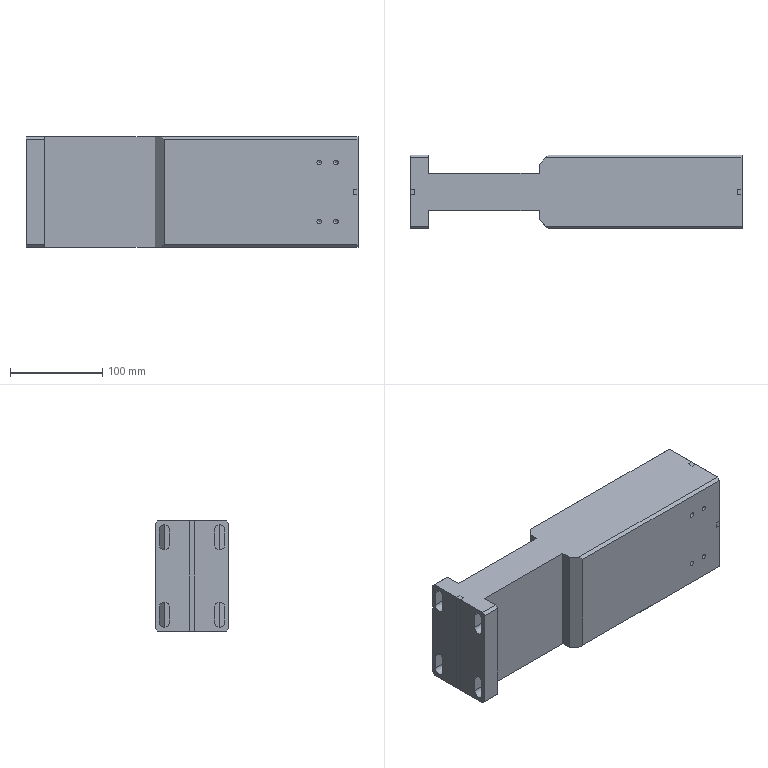CAM job | NX | 3+2 milling, drilling | part box 360 x 80 x 120 mm | stock box 365 x 85 x 125 mm
Tools:
number,name,description,diameter,corner_radius,flute_length,length,flutes
4,D4,平底铣刀-粗,4.0,0.0,25.0,75.0,2
6,D6,平底铣刀-粗,6.0,0.0,25.0,75.0,2
9,D10,平底铣刀-粗,10.0,0.0,35.0,75.0,2
17,D16,平底铣刀-粗,16.0,0.0,50.0,75.0,2
11,D4-J,平底铣刀-精,4.0,0.0,50.0,75.0,2
7,D6-J,平底铣刀-精,6.0,0.0,25.0,75.0,2
10,D10-J,平底铣刀-精,10.0,0.0,35.0,75.0,2
18,D16-J,平底铣刀-精,16.0,0.0,50.0,75.0,2
1,D80R0.8飞刀,圆鼻刀-粗,80.0,0.8,50.0,75.0,2
19,D6R0.5-J,圆鼻刀-精,6.0,0.5,50.0,75.0,2
1,D80R0.8飞刀-J,圆鼻刀-精,80.0,0.8,50.0,75.0,2
2,D6倒角刀,倒角刀,6.0,0.0,3.0,25.0,2
22,M6X1.0,丝锥,5.0,0.0,35.0,50.0,2
18,M8X1.25,丝锥,6.8,0.0,35.0,50.0,2
15,ZT5.1,钻头,5.1,0.0,35.0,50.0,2
17,ZT6.9,Drilling Tool,6.9,0.0,35.0,50.0,2
Operations:
program,operation,operation_type,tool,method,geometry_group,spindle_rpm,surface_speed,feed_per_tooth,feed_cut,feed_plunge,cut_length_mm,path_length_mm,cut_time_min,machine_time_min
D,FLOORWALL_HELIXROUGH-MID_COPY,VolumeBased25DMillingOperation,D6,LAYERROUGH-DEPTHK-STEPG,W-D,8000.0,150.796,0.125,2000.0,100.0,8133.076,8800.416,4.066,4.133
D,FLOORWALL_LAYERROUGH-MID_COPY_COPY,VolumeBased25DMillingOperation,D4,LAYERROUGH-DEPTHK-STEPG,W-D,8000.0,100.528,0.125,2000.0,100.0,4528.8,4610.955,2.264,2.273
D,PLANARDEBURR6X45L_COPY_2,SurfaceContour,D6倒角刀,CONTOUR_CHAMFER-DEPTH0-STEPG,W-D,6500.0,122.519,0.1154,1500.0,100.0,896.525,1415.715,0.5977,0.6496
D,FLOORWALL_HELIXFINISH-MID_COPY,VolumeBased25DMillingOperation,D6-J,HELIXFINISH-DEPTHK-STEPG,W-D,8000.0,150.792,0.0625,1000.0,100.0,1193.037,1874.777,1.193,1.261
D,FLOORWALL_FINISHSIDE-MID-SELFLOOR_COPY_1_COPY,VolumeBased25DMillingOperation,D4-J,SIDEFINISH-DEPTHK-STEPG,W-D,8000.0,100.528,0.05,800.0,100.0,255.552,283.553,0.3194,0.3222
C,FLOORWALL_LAYERROUGH-MID_COPY,VolumeBased25DMillingOperation,D4,LAYERROUGH-DEPTHK-STEPG,W-C,8000.0,100.528,0.125,2000.0,100.0,7575.2,7718.555,3.788,3.802
C,SPOT-DEPTH0.8_3,Operation,D6倒角刀,NONE,W-C,8000.0,150.796,0.0312,500.0,90.0,7.2,297.422,0.0144,0.0434
C,NG_BLINDTAPERHOLE-M8TAPDRILL,Operation,ZT6.9,NONE,W-C,2200.0,46.998,0.0341,150.0,90.0,104.0,491.022,0.6933,0.732
C,MILLCHAMFER_3,PlanarMilling,D6倒角刀,METHOD,W-C,8000.0,150.796,0.0375,600.0,100.0,97.605,564.85,0.1627,0.2094
C,PLANARDEBURR6X45L_COPY_1,SurfaceContour,D6倒角刀,CONTOUR_CHAMFER-DEPTH0-STEPG,W-C,6500.0,122.519,0.1154,1500.0,100.0,860.257,1354.65,0.5735,0.6229
C,BLINDTAPERHOLE-TAPM8,Operation,M8X1.25,METHOD,W-C,500.0,10.681,0.0013,1.25,90.0,81.0,445.022,64.8,64.836
C,FLOORWALL_FINISHSIDE-MID-SELFLOOR_COPY_1,VolumeBased25DMillingOperation,D4-J,SIDEFINISH-DEPTHK-STEPG,W-C,8000.0,100.528,0.05,800.0,100.0,421.329,449.33,0.5267,0.5295
B,FLOORWALL_FACEMILLROUGH_COPY,VolumeBased25DMillingOperation,D80R0.8飞刀,LAYERROUGH-DEPTHK-STEPG,W-B,2800.0,703.696,0.5357,3000.0,100.0,8697.187,9307.757,2.899,2.96
B,FLOORWALL_FACEMILLFINISH_COPY,VolumeBased25DMillingOperation,D80R0.8飞刀-J,SIDEFINISH-DEPTHK-STEPG,W-B,4000.0,1005.28,0.125,1000.0,100.0,1399.584,1495.584,1.4,1.409
B,CAVITY_ROUGH-MID_COPY_COPY,CavityMilling,D10,LAYERROUGH-DEPTHK-STEPG,W-B,8000.0,251.32,0.25,4000.0,100.0,75619.731,78566.63,18.905,19.34
B,SPOT-DEPTH0.8_2,Operation,D6倒角刀,NONE,W-B,3000.0,56.0,0.01,60.0,90.0,7.2,217.463,0.12,0.141
B,NG_BLINDTAPERHOLE-M6TAPDRILL_2,Operation,ZT5.1,NONE,W-B,1200.0,19.227,0.125,300.0,90.0,80.0,363.063,0.2667,0.295
B,ZLEVEL_FINISHZIGZAGCONTOUR_COPY_COPY_1,ZLevelMilling,D6R0.5-J,ZLEVELCONTOUR-DEPTHK-STEPG,W-B,8000.0,150.796,0.2812,4500.0,100.0,18105.798,18144.868,4.024,4.027
B,ZLEVEL_FINISHZIGZAGCONTOUR_COPY_COPY_1_COPY,ZLevelMilling,D6R0.5-J,ZLEVELCONTOUR-DEPTHK-STEPG,W-B,8000.0,150.796,0.2812,4500.0,100.0,23657.928,24309.159,5.257,5.322
B,MILLCHAMFER_2,PlanarMilling,D6倒角刀,METHOD,W-B,6500.0,122.522,0.0462,600.0,100.0,79.753,584.585,0.1329,0.1834
B,PLANARDEBURR6X45L_COPY,SurfaceContour,D6倒角刀,CONTOUR_CHAMFER-DEPTH0-STEPG,W-B,6500.0,122.519,0.1154,1500.0,100.0,692.088,1865.998,0.4614,0.5788
B,BLINDTAPERHOLE-TAPM6_2,Operation,M6X1.0,METHOD,W-B,400.0,6.283,0.0013,1.0,90.0,62.0,327.063,62.0,62.026
B,FLOORWALL_FINISHFLOOR-MID_COPY,VolumeBased25DMillingOperation,D10-J,FINISHSTEPDEPTHOFF,W-B,8000.0,251.32,0.0625,1000.0,100.0,2907.07,2973.07,2.907,2.914
B,FLOORWALL_FINISHSIDE-MID-SELFLOOR_COPY,VolumeBased25DMillingOperation,D10-J,SIDEFINISH-DEPTHK-STEPG,W-B,8000.0,251.32,0.0625,1000.0,100.0,277.362,449.964,0.2774,0.2946
A,TOPFACE,FaceMilling,D80R0.8飞刀,SIDEFINISH-DEPTHK-STEPG,W-A,4500.0,1385.0,0.1667,1500.0,100.0,1434.0,1530.0,0.956,0.9656
A,PROFILE_ROUGH_2,VolumeBased25DMillingOperation,D16,METHOD,W-A,6000.0,301.593,0.5,6000.0,80.0,103112.699,103291.199,17.185,17.203
A,CAVITY_ROUGH-MID_COPY,CavityMilling,D10,LAYERROUGH-DEPTHK-STEPG,W-A,8000.0,251.32,0.25,4000.0,100.0,88981.094,92438.493,22.245,22.756
A,SPOT-DEPTH0.8,Operation,D6倒角刀,NONE,W-A,8000.0,150.796,0.0312,500.0,90.0,7.2,217.463,0.0144,0.0354
A,NG_BLINDTAPERHOLE-M6TAPDRILL,Operation,ZT5.1,NONE,W-A,2500.0,39.27,0.03,150.0,90.0,80.0,363.063,0.5333,0.5616
A,ZLEVEL_FINISHZIGZAGCONTOUR_COPY,ZLevelMilling,D6R0.5-J,ZLEVELCONTOUR-DEPTHK-STEPG,W-A,8000.0,150.796,0.2812,4500.0,100.0,18105.804,18137.45,4.024,4.027
A,ZLEVEL_FINISHZIGZAGCONTOUR_COPY_COPY,ZLevelMilling,D6R0.5-J,ZLEVELCONTOUR-DEPTHK-STEPG,W-A,8000.0,150.796,0.2812,4500.0,100.0,23657.929,24279.463,5.257,5.319
A,SOLIDONLY,SurfaceContour,D6倒角刀,METHOD,W-A,8000.0,150.796,0.1875,3000.0,100.0,673.495,1900.463,0.2245,0.3472
A,MILLCHAMFER_1,PlanarMilling,D6倒角刀,METHOD,W-A,8000.0,150.796,0.0375,600.0,100.0,75.821,582.245,0.1264,0.177
A,BLINDTAPERHOLE-TAPM6,Operation,M6X1.0,METHOD,W-A,500.0,7.854,0.001,1.0,90.0,64.0,331.063,64.0,64.027
A,FLOORFINISH_1,VolumeBased25DMillingOperation,D10-J,METHOD,W-A,9000.0,169.646,0.0833,1500.0,100.0,2237.2,2376.2,1.492,1.505
A,FLOORSIDEFINISH_3,VolumeBased25DMillingOperation,D10-J,METHOD,W-A,9000.0,169.646,0.0833,1500.0,100.0,800.05,2139.41,0.5334,0.6673
A,PROFILE_SEMIFINISH_2,VolumeBased25DMillingOperation,D16-J,METHOD,W-A,9000.0,169.646,0.0667,1200.0,100.0,7106.76,8454.822,5.922,6.057